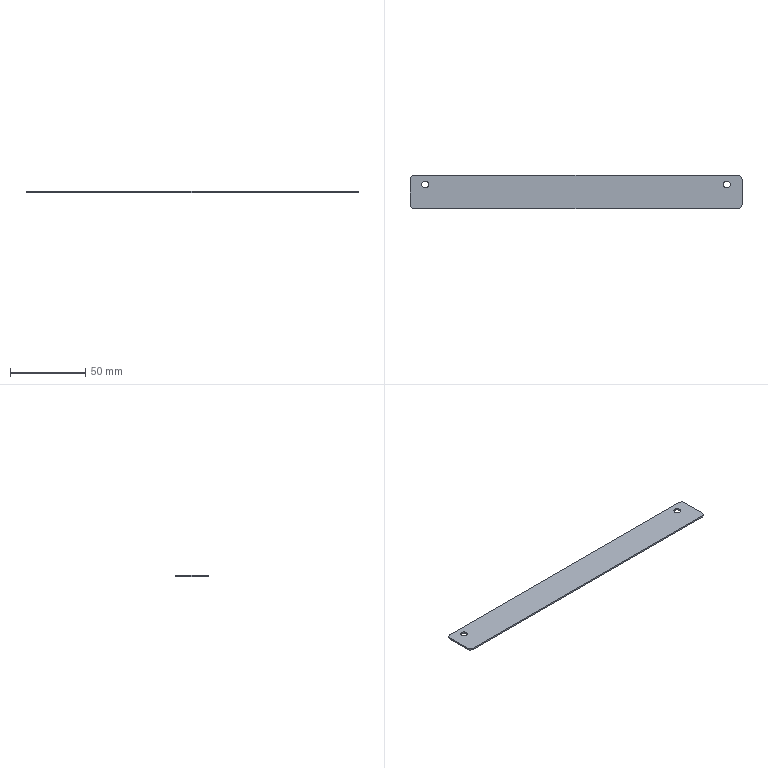Part | STEP file | TY.NE-0002-01-017A Keyboard press block-dddeger | 1 solid | 14 faces | box 220 x 22 x 1 mm | volume 4800 mm3 | cylinder 8 | plane 6 | commonest cylinder face diameters 4.5 x4 6 x4
STEP:
#1=CARTESIAN_POINT('',(0.,0.,0.));
#2=DIRECTION('',(0.,0.,1.));
#3=DIRECTION('',(1.,0.,0.));
#4=AXIS2_PLACEMENT_3D('',#1,#2,#3);
#5=CARTESIAN_POINT('',(102.25,5.,-1.));
#6=VERTEX_POINT('',#5);
#7=CARTESIAN_POINT('',(102.25,5.,0.));
#8=VERTEX_POINT('',#7);
#9=CARTESIAN_POINT('',(102.25,5.,-1.));
#10=DIRECTION('',(0.,0.,1.));
#11=VECTOR('',#10,1.);
#12=LINE('',#9,#11);
#13=CARTESIAN_POINT('',(100.,5.,-1.));
#14=DIRECTION('',(0.,0.,1.));
#15=DIRECTION('',(1.,0.,0.));
#16=AXIS2_PLACEMENT_3D('',#13,#14,#15);
#17=CYLINDRICAL_SURFACE('',#16,2.25);
#18=CARTESIAN_POINT('',(6.283,0.));
#19=DIRECTION('',(0.,1.));
#20=VECTOR('',#19,1.);
#21=LINE('',#18,#20);
#22=(GEOMETRIC_REPRESENTATION_CONTEXT(2)PARAMETRIC_REPRESENTATION_CONTEXT()REPRESENTATION_CONTEXT('',''));
#23=DEFINITIONAL_REPRESENTATION('',(#21),#22);
#24=PCURVE('',#17,#23);
#25=CARTESIAN_POINT('',(100.,5.,-1.));
#26=DIRECTION('',(0.,0.,1.));
#27=DIRECTION('',(1.,0.,0.));
#28=AXIS2_PLACEMENT_3D('',#25,#26,#27);
#29=CYLINDRICAL_SURFACE('',#28,2.25);
#30=CARTESIAN_POINT('',(0.,0.));
#31=DIRECTION('',(0.,1.));
#32=VECTOR('',#31,1.);
#33=LINE('',#30,#32);
#34=(GEOMETRIC_REPRESENTATION_CONTEXT(2)PARAMETRIC_REPRESENTATION_CONTEXT()REPRESENTATION_CONTEXT('',''));
#35=DEFINITIONAL_REPRESENTATION('',(#33),#34);
#36=PCURVE('',#29,#35);
#37=SURFACE_CURVE('',#12,(#24,#36),.PCURVE_S1.);
#38=EDGE_CURVE('',#6,#8,#37,.T.);
#39=ORIENTED_EDGE('',*,*,#38,.T.);
#40=CARTESIAN_POINT('',(97.75,5.,0.));
#41=VERTEX_POINT('',#40);
#42=CARTESIAN_POINT('',(100.,5.,0.));
#43=DIRECTION('',(0.,0.,1.));
#44=DIRECTION('',(-1.,0.,0.));
#45=AXIS2_PLACEMENT_3D('',#42,#43,#44);
#46=CIRCLE('',#45,2.25);
#47=CARTESIAN_POINT('',(3.142,1.));
#48=DIRECTION('',(1.,0.));
#49=VECTOR('',#48,1.);
#50=LINE('',#47,#49);
#51=(GEOMETRIC_REPRESENTATION_CONTEXT(2)PARAMETRIC_REPRESENTATION_CONTEXT()REPRESENTATION_CONTEXT('',''));
#52=DEFINITIONAL_REPRESENTATION('',(#50),#51);
#53=PCURVE('',#17,#52);
#54=CARTESIAN_POINT('',(0.,0.,0.));
#55=DIRECTION('',(0.,0.,1.));
#56=DIRECTION('',(1.,0.,0.));
#57=AXIS2_PLACEMENT_3D('',#54,#55,#56);
#58=PLANE('',#57);
#59=CARTESIAN_POINT('',(100.,5.));
#60=DIRECTION('',(-1.,0.));
#61=AXIS2_PLACEMENT_2D('',#59,#60);
#62=CIRCLE('',#61,2.25);
#63=(GEOMETRIC_REPRESENTATION_CONTEXT(2)PARAMETRIC_REPRESENTATION_CONTEXT()REPRESENTATION_CONTEXT('',''));
#64=DEFINITIONAL_REPRESENTATION('',(#62),#63);
#65=PCURVE('',#58,#64);
#66=SURFACE_CURVE('',#46,(#53,#65),.PCURVE_S1.);
#67=EDGE_CURVE('',#41,#8,#66,.T.);
#68=ORIENTED_EDGE('',*,*,#67,.F.);
#69=CARTESIAN_POINT('',(97.75,5.,-1.));
#70=VERTEX_POINT('',#69);
#71=CARTESIAN_POINT('',(97.75,5.,-1.));
#72=DIRECTION('',(0.,0.,1.));
#73=VECTOR('',#72,1.);
#74=LINE('',#71,#73);
#75=CARTESIAN_POINT('',(3.142,0.));
#76=DIRECTION('',(0.,1.));
#77=VECTOR('',#76,1.);
#78=LINE('',#75,#77);
#79=(GEOMETRIC_REPRESENTATION_CONTEXT(2)PARAMETRIC_REPRESENTATION_CONTEXT()REPRESENTATION_CONTEXT('',''));
#80=DEFINITIONAL_REPRESENTATION('',(#78),#79);
#81=PCURVE('',#17,#80);
#82=CARTESIAN_POINT('',(3.142,0.));
#83=DIRECTION('',(0.,1.));
#84=VECTOR('',#83,1.);
#85=LINE('',#82,#84);
#86=(GEOMETRIC_REPRESENTATION_CONTEXT(2)PARAMETRIC_REPRESENTATION_CONTEXT()REPRESENTATION_CONTEXT('',''));
#87=DEFINITIONAL_REPRESENTATION('',(#85),#86);
#88=PCURVE('',#29,#87);
#89=SURFACE_CURVE('',#74,(#81,#88),.PCURVE_S1.);
#90=EDGE_CURVE('',#70,#41,#89,.T.);
#91=ORIENTED_EDGE('',*,*,#90,.F.);
#92=CARTESIAN_POINT('',(100.,5.,-1.));
#93=DIRECTION('',(0.,0.,1.));
#94=DIRECTION('',(-1.,0.,0.));
#95=AXIS2_PLACEMENT_3D('',#92,#93,#94);
#96=CIRCLE('',#95,2.25);
#97=CARTESIAN_POINT('',(3.142,0.));
#98=DIRECTION('',(1.,0.));
#99=VECTOR('',#98,1.);
#100=LINE('',#97,#99);
#101=(GEOMETRIC_REPRESENTATION_CONTEXT(2)PARAMETRIC_REPRESENTATION_CONTEXT()REPRESENTATION_CONTEXT('',''));
#102=DEFINITIONAL_REPRESENTATION('',(#100),#101);
#103=PCURVE('',#17,#102);
#104=CARTESIAN_POINT('',(0.,0.,-1.));
#105=DIRECTION('',(0.,0.,1.));
#106=DIRECTION('',(1.,0.,0.));
#107=AXIS2_PLACEMENT_3D('',#104,#105,#106);
#108=PLANE('',#107);
#109=CARTESIAN_POINT('',(100.,5.));
#110=DIRECTION('',(-1.,0.));
#111=AXIS2_PLACEMENT_2D('',#109,#110);
#112=CIRCLE('',#111,2.25);
#113=(GEOMETRIC_REPRESENTATION_CONTEXT(2)PARAMETRIC_REPRESENTATION_CONTEXT()REPRESENTATION_CONTEXT('',''));
#114=DEFINITIONAL_REPRESENTATION('',(#112),#113);
#115=PCURVE('',#108,#114);
#116=SURFACE_CURVE('',#96,(#103,#115),.PCURVE_S1.);
#117=EDGE_CURVE('',#70,#6,#116,.T.);
#118=ORIENTED_EDGE('',*,*,#117,.T.);
#119=EDGE_LOOP('',(#39,#68,#91,#118));
#120=FACE_BOUND('',#119,.F.);
#121=ADVANCED_FACE('',(#120),#17,.F.);
#122=CARTESIAN_POINT('',(-97.75,5.,-1.));
#123=VERTEX_POINT('',#122);
#124=CARTESIAN_POINT('',(-97.75,5.,0.));
#125=VERTEX_POINT('',#124);
#126=CARTESIAN_POINT('',(-97.75,5.,-1.));
#127=DIRECTION('',(0.,0.,1.));
#128=VECTOR('',#127,1.);
#129=LINE('',#126,#128);
#130=CARTESIAN_POINT('',(-100.,5.,-1.));
#131=DIRECTION('',(0.,0.,1.));
#132=DIRECTION('',(1.,0.,0.));
#133=AXIS2_PLACEMENT_3D('',#130,#131,#132);
#134=CYLINDRICAL_SURFACE('',#133,2.25);
#135=CARTESIAN_POINT('',(6.283,0.));
#136=DIRECTION('',(0.,1.));
#137=VECTOR('',#136,1.);
#138=LINE('',#135,#137);
#139=(GEOMETRIC_REPRESENTATION_CONTEXT(2)PARAMETRIC_REPRESENTATION_CONTEXT()REPRESENTATION_CONTEXT('',''));
#140=DEFINITIONAL_REPRESENTATION('',(#138),#139);
#141=PCURVE('',#134,#140);
#142=CARTESIAN_POINT('',(-100.,5.,-1.));
#143=DIRECTION('',(0.,0.,1.));
#144=DIRECTION('',(1.,0.,0.));
#145=AXIS2_PLACEMENT_3D('',#142,#143,#144);
#146=CYLINDRICAL_SURFACE('',#145,2.25);
#147=CARTESIAN_POINT('',(0.,0.));
#148=DIRECTION('',(0.,1.));
#149=VECTOR('',#148,1.);
#150=LINE('',#147,#149);
#151=(GEOMETRIC_REPRESENTATION_CONTEXT(2)PARAMETRIC_REPRESENTATION_CONTEXT()REPRESENTATION_CONTEXT('',''));
#152=DEFINITIONAL_REPRESENTATION('',(#150),#151);
#153=PCURVE('',#146,#152);
#154=SURFACE_CURVE('',#129,(#141,#153),.PCURVE_S1.);
#155=EDGE_CURVE('',#123,#125,#154,.T.);
#156=ORIENTED_EDGE('',*,*,#155,.T.);
#157=CARTESIAN_POINT('',(-102.25,5.,0.));
#158=VERTEX_POINT('',#157);
#159=CARTESIAN_POINT('',(-100.,5.,0.));
#160=DIRECTION('',(0.,0.,1.));
#161=DIRECTION('',(1.,0.,0.));
#162=AXIS2_PLACEMENT_3D('',#159,#160,#161);
#163=CIRCLE('',#162,2.25);
#164=CARTESIAN_POINT('',(0.,1.));
#165=DIRECTION('',(1.,0.));
#166=VECTOR('',#165,1.);
#167=LINE('',#164,#166);
#168=(GEOMETRIC_REPRESENTATION_CONTEXT(2)PARAMETRIC_REPRESENTATION_CONTEXT()REPRESENTATION_CONTEXT('',''));
#169=DEFINITIONAL_REPRESENTATION('',(#167),#168);
#170=PCURVE('',#134,#169);
#171=CARTESIAN_POINT('',(-100.,5.));
#172=DIRECTION('',(1.,0.));
#173=AXIS2_PLACEMENT_2D('',#171,#172);
#174=CIRCLE('',#173,2.25);
#175=(GEOMETRIC_REPRESENTATION_CONTEXT(2)PARAMETRIC_REPRESENTATION_CONTEXT()REPRESENTATION_CONTEXT('',''));
#176=DEFINITIONAL_REPRESENTATION('',(#174),#175);
#177=PCURVE('',#58,#176);
#178=SURFACE_CURVE('',#163,(#170,#177),.PCURVE_S1.);
#179=EDGE_CURVE('',#158,#125,#178,.T.);
#180=ORIENTED_EDGE('',*,*,#179,.F.);
#181=CARTESIAN_POINT('',(-102.25,5.,-1.));
#182=VERTEX_POINT('',#181);
#183=CARTESIAN_POINT('',(-102.25,5.,-1.));
#184=DIRECTION('',(0.,0.,1.));
#185=VECTOR('',#184,1.);
#186=LINE('',#183,#185);
#187=CARTESIAN_POINT('',(3.142,0.));
#188=DIRECTION('',(0.,1.));
#189=VECTOR('',#188,1.);
#190=LINE('',#187,#189);
#191=(GEOMETRIC_REPRESENTATION_CONTEXT(2)PARAMETRIC_REPRESENTATION_CONTEXT()REPRESENTATION_CONTEXT('',''));
#192=DEFINITIONAL_REPRESENTATION('',(#190),#191);
#193=PCURVE('',#134,#192);
#194=CARTESIAN_POINT('',(3.142,0.));
#195=DIRECTION('',(0.,1.));
#196=VECTOR('',#195,1.);
#197=LINE('',#194,#196);
#198=(GEOMETRIC_REPRESENTATION_CONTEXT(2)PARAMETRIC_REPRESENTATION_CONTEXT()REPRESENTATION_CONTEXT('',''));
#199=DEFINITIONAL_REPRESENTATION('',(#197),#198);
#200=PCURVE('',#146,#199);
#201=SURFACE_CURVE('',#186,(#193,#200),.PCURVE_S1.);
#202=EDGE_CURVE('',#182,#158,#201,.T.);
#203=ORIENTED_EDGE('',*,*,#202,.F.);
#204=CARTESIAN_POINT('',(-100.,5.,-1.));
#205=DIRECTION('',(0.,0.,1.));
#206=DIRECTION('',(1.,0.,0.));
#207=AXIS2_PLACEMENT_3D('',#204,#205,#206);
#208=CIRCLE('',#207,2.25);
#209=CARTESIAN_POINT('',(0.,0.));
#210=DIRECTION('',(1.,0.));
#211=VECTOR('',#210,1.);
#212=LINE('',#209,#211);
#213=(GEOMETRIC_REPRESENTATION_CONTEXT(2)PARAMETRIC_REPRESENTATION_CONTEXT()REPRESENTATION_CONTEXT('',''));
#214=DEFINITIONAL_REPRESENTATION('',(#212),#213);
#215=PCURVE('',#134,#214);
#216=CARTESIAN_POINT('',(-100.,5.));
#217=DIRECTION('',(1.,0.));
#218=AXIS2_PLACEMENT_2D('',#216,#217);
#219=CIRCLE('',#218,2.25);
#220=(GEOMETRIC_REPRESENTATION_CONTEXT(2)PARAMETRIC_REPRESENTATION_CONTEXT()REPRESENTATION_CONTEXT('',''));
#221=DEFINITIONAL_REPRESENTATION('',(#219),#220);
#222=PCURVE('',#108,#221);
#223=SURFACE_CURVE('',#208,(#215,#222),.PCURVE_S1.);
#224=EDGE_CURVE('',#182,#123,#223,.T.);
#225=ORIENTED_EDGE('',*,*,#224,.T.);
#226=EDGE_LOOP('',(#156,#180,#203,#225));
#227=FACE_BOUND('',#226,.F.);
#228=ADVANCED_FACE('',(#227),#134,.F.);
#229=CARTESIAN_POINT('',(-110.,8.,-1.));
#230=VERTEX_POINT('',#229);
#231=CARTESIAN_POINT('',(-110.,-8.,-1.));
#232=VERTEX_POINT('',#231);
#233=CARTESIAN_POINT('',(-110.,-11.,-1.));
#234=DIRECTION('',(0.,-1.,0.));
#235=VECTOR('',#234,1.);
#236=LINE('',#233,#235);
#237=CARTESIAN_POINT('',(-110.,-11.,-1.));
#238=DIRECTION('',(-1.,0.,0.));
#239=DIRECTION('',(0.,0.,1.));
#240=AXIS2_PLACEMENT_3D('',#237,#238,#239);
#241=PLANE('',#240);
#242=CARTESIAN_POINT('',(0.,0.));
#243=DIRECTION('',(0.,-1.));
#244=VECTOR('',#243,1.);
#245=LINE('',#242,#244);
#246=(GEOMETRIC_REPRESENTATION_CONTEXT(2)PARAMETRIC_REPRESENTATION_CONTEXT()REPRESENTATION_CONTEXT('',''));
#247=DEFINITIONAL_REPRESENTATION('',(#245),#246);
#248=PCURVE('',#241,#247);
#249=CARTESIAN_POINT('',(-110.,-11.));
#250=DIRECTION('',(0.,-1.));
#251=VECTOR('',#250,1.);
#252=LINE('',#249,#251);
#253=(GEOMETRIC_REPRESENTATION_CONTEXT(2)PARAMETRIC_REPRESENTATION_CONTEXT()REPRESENTATION_CONTEXT('',''));
#254=DEFINITIONAL_REPRESENTATION('',(#252),#253);
#255=PCURVE('',#108,#254);
#256=SURFACE_CURVE('',#236,(#248,#255),.PCURVE_S1.);
#257=EDGE_CURVE('',#230,#232,#256,.T.);
#258=ORIENTED_EDGE('',*,*,#257,.T.);
#259=CARTESIAN_POINT('',(-110.,-8.,0.));
#260=VERTEX_POINT('',#259);
#261=CARTESIAN_POINT('',(-110.,-8.,-1.));
#262=DIRECTION('',(0.,0.,1.));
#263=VECTOR('',#262,1.);
#264=LINE('',#261,#263);
#265=CARTESIAN_POINT('',(0.,3.));
#266=DIRECTION('',(1.,0.));
#267=VECTOR('',#266,1.);
#268=LINE('',#265,#267);
#269=(GEOMETRIC_REPRESENTATION_CONTEXT(2)PARAMETRIC_REPRESENTATION_CONTEXT()REPRESENTATION_CONTEXT('',''));
#270=DEFINITIONAL_REPRESENTATION('',(#268),#269);
#271=PCURVE('',#241,#270);
#272=CARTESIAN_POINT('',(-107.,-8.,-1.));
#273=DIRECTION('',(0.,0.,1.));
#274=DIRECTION('',(1.,0.,0.));
#275=AXIS2_PLACEMENT_3D('',#272,#273,#274);
#276=CYLINDRICAL_SURFACE('',#275,3.);
#277=CARTESIAN_POINT('',(3.142,0.));
#278=DIRECTION('',(0.,1.));
#279=VECTOR('',#278,1.);
#280=LINE('',#277,#279);
#281=(GEOMETRIC_REPRESENTATION_CONTEXT(2)PARAMETRIC_REPRESENTATION_CONTEXT()REPRESENTATION_CONTEXT('',''));
#282=DEFINITIONAL_REPRESENTATION('',(#280),#281);
#283=PCURVE('',#276,#282);
#284=SURFACE_CURVE('',#264,(#271,#283),.PCURVE_S1.);
#285=EDGE_CURVE('',#232,#260,#284,.T.);
#286=ORIENTED_EDGE('',*,*,#285,.T.);
#287=CARTESIAN_POINT('',(-110.,8.,0.));
#288=VERTEX_POINT('',#287);
#289=CARTESIAN_POINT('',(-110.,-11.,0.));
#290=DIRECTION('',(0.,-1.,0.));
#291=VECTOR('',#290,1.);
#292=LINE('',#289,#291);
#293=CARTESIAN_POINT('',(1.,0.));
#294=DIRECTION('',(0.,-1.));
#295=VECTOR('',#294,1.);
#296=LINE('',#293,#295);
#297=(GEOMETRIC_REPRESENTATION_CONTEXT(2)PARAMETRIC_REPRESENTATION_CONTEXT()REPRESENTATION_CONTEXT('',''));
#298=DEFINITIONAL_REPRESENTATION('',(#296),#297);
#299=PCURVE('',#241,#298);
#300=CARTESIAN_POINT('',(-110.,-11.));
#301=DIRECTION('',(0.,-1.));
#302=VECTOR('',#301,1.);
#303=LINE('',#300,#302);
#304=(GEOMETRIC_REPRESENTATION_CONTEXT(2)PARAMETRIC_REPRESENTATION_CONTEXT()REPRESENTATION_CONTEXT('',''));
#305=DEFINITIONAL_REPRESENTATION('',(#303),#304);
#306=PCURVE('',#58,#305);
#307=SURFACE_CURVE('',#292,(#299,#306),.PCURVE_S1.);
#308=EDGE_CURVE('',#288,#260,#307,.T.);
#309=ORIENTED_EDGE('',*,*,#308,.F.);
#310=CARTESIAN_POINT('',(-110.,8.,-1.));
#311=DIRECTION('',(0.,0.,-1.));
#312=VECTOR('',#311,1.);
#313=LINE('',#310,#312);
#314=CARTESIAN_POINT('',(0.,19.));
#315=DIRECTION('',(-1.,0.));
#316=VECTOR('',#315,1.);
#317=LINE('',#314,#316);
#318=(GEOMETRIC_REPRESENTATION_CONTEXT(2)PARAMETRIC_REPRESENTATION_CONTEXT()REPRESENTATION_CONTEXT('',''));
#319=DEFINITIONAL_REPRESENTATION('',(#317),#318);
#320=PCURVE('',#241,#319);
#321=CARTESIAN_POINT('',(-107.,8.,-1.));
#322=DIRECTION('',(0.,0.,1.));
#323=DIRECTION('',(1.,0.,0.));
#324=AXIS2_PLACEMENT_3D('',#321,#322,#323);
#325=CYLINDRICAL_SURFACE('',#324,3.);
#326=CARTESIAN_POINT('',(3.142,0.));
#327=DIRECTION('',(0.,-1.));
#328=VECTOR('',#327,1.);
#329=LINE('',#326,#328);
#330=(GEOMETRIC_REPRESENTATION_CONTEXT(2)PARAMETRIC_REPRESENTATION_CONTEXT()REPRESENTATION_CONTEXT('',''));
#331=DEFINITIONAL_REPRESENTATION('',(#329),#330);
#332=PCURVE('',#325,#331);
#333=SURFACE_CURVE('',#313,(#320,#332),.PCURVE_S1.);
#334=EDGE_CURVE('',#288,#230,#333,.T.);
#335=ORIENTED_EDGE('',*,*,#334,.T.);
#336=EDGE_LOOP('',(#258,#286,#309,#335));
#337=FACE_BOUND('',#336,.T.);
#338=ADVANCED_FACE('',(#337),#241,.T.);
#339=CARTESIAN_POINT('',(107.,11.,-1.));
#340=VERTEX_POINT('',#339);
#341=CARTESIAN_POINT('',(-107.,11.,-1.));
#342=VERTEX_POINT('',#341);
#343=CARTESIAN_POINT('',(110.,11.,-1.));
#344=DIRECTION('',(-1.,0.,0.));
#345=VECTOR('',#344,1.);
#346=LINE('',#343,#345);
#347=CARTESIAN_POINT('',(110.,11.,-1.));
#348=DIRECTION('',(0.,1.,0.));
#349=DIRECTION('',(-1.,0.,0.));
#350=AXIS2_PLACEMENT_3D('',#347,#348,#349);
#351=PLANE('',#350);
#352=CARTESIAN_POINT('',(0.,0.));
#353=DIRECTION('',(1.,0.));
#354=VECTOR('',#353,1.);
#355=LINE('',#352,#354);
#356=(GEOMETRIC_REPRESENTATION_CONTEXT(2)PARAMETRIC_REPRESENTATION_CONTEXT()REPRESENTATION_CONTEXT('',''));
#357=DEFINITIONAL_REPRESENTATION('',(#355),#356);
#358=PCURVE('',#351,#357);
#359=CARTESIAN_POINT('',(110.,11.));
#360=DIRECTION('',(-1.,0.));
#361=VECTOR('',#360,1.);
#362=LINE('',#359,#361);
#363=(GEOMETRIC_REPRESENTATION_CONTEXT(2)PARAMETRIC_REPRESENTATION_CONTEXT()REPRESENTATION_CONTEXT('',''));
#364=DEFINITIONAL_REPRESENTATION('',(#362),#363);
#365=PCURVE('',#108,#364);
#366=SURFACE_CURVE('',#346,(#358,#365),.PCURVE_S1.);
#367=EDGE_CURVE('',#340,#342,#366,.T.);
#368=ORIENTED_EDGE('',*,*,#367,.T.);
#369=CARTESIAN_POINT('',(-107.,11.,0.));
#370=VERTEX_POINT('',#369);
#371=CARTESIAN_POINT('',(-107.,11.,-1.));
#372=DIRECTION('',(0.,0.,1.));
#373=VECTOR('',#372,1.);
#374=LINE('',#371,#373);
#375=CARTESIAN_POINT('',(217.,0.));
#376=DIRECTION('',(0.,1.));
#377=VECTOR('',#376,1.);
#378=LINE('',#375,#377);
#379=(GEOMETRIC_REPRESENTATION_CONTEXT(2)PARAMETRIC_REPRESENTATION_CONTEXT()REPRESENTATION_CONTEXT('',''));
#380=DEFINITIONAL_REPRESENTATION('',(#378),#379);
#381=PCURVE('',#351,#380);
#382=CARTESIAN_POINT('',(1.571,0.));
#383=DIRECTION('',(0.,1.));
#384=VECTOR('',#383,1.);
#385=LINE('',#382,#384);
#386=(GEOMETRIC_REPRESENTATION_CONTEXT(2)PARAMETRIC_REPRESENTATION_CONTEXT()REPRESENTATION_CONTEXT('',''));
#387=DEFINITIONAL_REPRESENTATION('',(#385),#386);
#388=PCURVE('',#325,#387);
#389=SURFACE_CURVE('',#374,(#381,#388),.PCURVE_S1.);
#390=EDGE_CURVE('',#342,#370,#389,.T.);
#391=ORIENTED_EDGE('',*,*,#390,.T.);
#392=CARTESIAN_POINT('',(107.,11.,0.));
#393=VERTEX_POINT('',#392);
#394=CARTESIAN_POINT('',(110.,11.,0.));
#395=DIRECTION('',(-1.,0.,0.));
#396=VECTOR('',#395,1.);
#397=LINE('',#394,#396);
#398=CARTESIAN_POINT('',(0.,1.));
#399=DIRECTION('',(1.,0.));
#400=VECTOR('',#399,1.);
#401=LINE('',#398,#400);
#402=(GEOMETRIC_REPRESENTATION_CONTEXT(2)PARAMETRIC_REPRESENTATION_CONTEXT()REPRESENTATION_CONTEXT('',''));
#403=DEFINITIONAL_REPRESENTATION('',(#401),#402);
#404=PCURVE('',#351,#403);
#405=CARTESIAN_POINT('',(110.,11.));
#406=DIRECTION('',(-1.,0.));
#407=VECTOR('',#406,1.);
#408=LINE('',#405,#407);
#409=(GEOMETRIC_REPRESENTATION_CONTEXT(2)PARAMETRIC_REPRESENTATION_CONTEXT()REPRESENTATION_CONTEXT('',''));
#410=DEFINITIONAL_REPRESENTATION('',(#408),#409);
#411=PCURVE('',#58,#410);
#412=SURFACE_CURVE('',#397,(#404,#411),.PCURVE_S1.);
#413=EDGE_CURVE('',#393,#370,#412,.T.);
#414=ORIENTED_EDGE('',*,*,#413,.F.);
#415=CARTESIAN_POINT('',(107.,11.,-1.));
#416=DIRECTION('',(0.,0.,-1.));
#417=VECTOR('',#416,1.);
#418=LINE('',#415,#417);
#419=CARTESIAN_POINT('',(3.,0.));
#420=DIRECTION('',(0.,-1.));
#421=VECTOR('',#420,1.);
#422=LINE('',#419,#421);
#423=(GEOMETRIC_REPRESENTATION_CONTEXT(2)PARAMETRIC_REPRESENTATION_CONTEXT()REPRESENTATION_CONTEXT('',''));
#424=DEFINITIONAL_REPRESENTATION('',(#422),#423);
#425=PCURVE('',#351,#424);
#426=CARTESIAN_POINT('',(107.,8.,-1.));
#427=DIRECTION('',(0.,0.,1.));
#428=DIRECTION('',(1.,0.,0.));
#429=AXIS2_PLACEMENT_3D('',#426,#427,#428);
#430=CYLINDRICAL_SURFACE('',#429,3.);
#431=CARTESIAN_POINT('',(1.571,0.));
#432=DIRECTION('',(0.,-1.));
#433=VECTOR('',#432,1.);
#434=LINE('',#431,#433);
#435=(GEOMETRIC_REPRESENTATION_CONTEXT(2)PARAMETRIC_REPRESENTATION_CONTEXT()REPRESENTATION_CONTEXT('',''));
#436=DEFINITIONAL_REPRESENTATION('',(#434),#435);
#437=PCURVE('',#430,#436);
#438=SURFACE_CURVE('',#418,(#425,#437),.PCURVE_S1.);
#439=EDGE_CURVE('',#393,#340,#438,.T.);
#440=ORIENTED_EDGE('',*,*,#439,.T.);
#441=EDGE_LOOP('',(#368,#391,#414,#440));
#442=FACE_BOUND('',#441,.T.);
#443=ADVANCED_FACE('',(#442),#351,.T.);
#444=CARTESIAN_POINT('',(110.,-8.,0.));
#445=VERTEX_POINT('',#444);
#446=CARTESIAN_POINT('',(110.,8.,0.));
#447=VERTEX_POINT('',#446);
#448=CARTESIAN_POINT('',(110.,-11.,0.));
#449=DIRECTION('',(0.,1.,0.));
#450=VECTOR('',#449,1.);
#451=LINE('',#448,#450);
#452=CARTESIAN_POINT('',(110.,-11.,-1.));
#453=DIRECTION('',(1.,0.,0.));
#454=DIRECTION('',(0.,0.,-1.));
#455=AXIS2_PLACEMENT_3D('',#452,#453,#454);
#456=PLANE('',#455);
#457=CARTESIAN_POINT('',(-1.,0.));
#458=DIRECTION('',(0.,1.));
#459=VECTOR('',#458,1.);
#460=LINE('',#457,#459);
#461=(GEOMETRIC_REPRESENTATION_CONTEXT(2)PARAMETRIC_REPRESENTATION_CONTEXT()REPRESENTATION_CONTEXT('',''));
#462=DEFINITIONAL_REPRESENTATION('',(#460),#461);
#463=PCURVE('',#456,#462);
#464=CARTESIAN_POINT('',(110.,-11.));
#465=DIRECTION('',(0.,1.));
#466=VECTOR('',#465,1.);
#467=LINE('',#464,#466);
#468=(GEOMETRIC_REPRESENTATION_CONTEXT(2)PARAMETRIC_REPRESENTATION_CONTEXT()REPRESENTATION_CONTEXT('',''));
#469=DEFINITIONAL_REPRESENTATION('',(#467),#468);
#470=PCURVE('',#58,#469);
#471=SURFACE_CURVE('',#451,(#463,#470),.PCURVE_S1.);
#472=EDGE_CURVE('',#445,#447,#471,.T.);
#473=ORIENTED_EDGE('',*,*,#472,.F.);
#474=CARTESIAN_POINT('',(110.,-8.,-1.));
#475=VERTEX_POINT('',#474);
#476=CARTESIAN_POINT('',(110.,-8.,-1.));
#477=DIRECTION('',(0.,0.,-1.));
#478=VECTOR('',#477,1.);
#479=LINE('',#476,#478);
#480=CARTESIAN_POINT('',(0.,3.));
#481=DIRECTION('',(1.,0.));
#482=VECTOR('',#481,1.);
#483=LINE('',#480,#482);
#484=(GEOMETRIC_REPRESENTATION_CONTEXT(2)PARAMETRIC_REPRESENTATION_CONTEXT()REPRESENTATION_CONTEXT('',''));
#485=DEFINITIONAL_REPRESENTATION('',(#483),#484);
#486=PCURVE('',#456,#485);
#487=CARTESIAN_POINT('',(107.,-8.,-1.));
#488=DIRECTION('',(0.,0.,1.));
#489=DIRECTION('',(1.,0.,0.));
#490=AXIS2_PLACEMENT_3D('',#487,#488,#489);
#491=CYLINDRICAL_SURFACE('',#490,3.);
#492=CARTESIAN_POINT('',(6.283,0.));
#493=DIRECTION('',(0.,-1.));
#494=VECTOR('',#493,1.);
#495=LINE('',#492,#494);
#496=(GEOMETRIC_REPRESENTATION_CONTEXT(2)PARAMETRIC_REPRESENTATION_CONTEXT()REPRESENTATION_CONTEXT('',''));
#497=DEFINITIONAL_REPRESENTATION('',(#495),#496);
#498=PCURVE('',#491,#497);
#499=SURFACE_CURVE('',#479,(#486,#498),.PCURVE_S1.);
#500=EDGE_CURVE('',#445,#475,#499,.T.);
#501=ORIENTED_EDGE('',*,*,#500,.T.);
#502=CARTESIAN_POINT('',(110.,8.,-1.));
#503=VERTEX_POINT('',#502);
#504=CARTESIAN_POINT('',(110.,-11.,-1.));
#505=DIRECTION('',(0.,1.,0.));
#506=VECTOR('',#505,1.);
#507=LINE('',#504,#506);
#508=CARTESIAN_POINT('',(0.,0.));
#509=DIRECTION('',(0.,1.));
#510=VECTOR('',#509,1.);
#511=LINE('',#508,#510);
#512=(GEOMETRIC_REPRESENTATION_CONTEXT(2)PARAMETRIC_REPRESENTATION_CONTEXT()REPRESENTATION_CONTEXT('',''));
#513=DEFINITIONAL_REPRESENTATION('',(#511),#512);
#514=PCURVE('',#456,#513);
#515=CARTESIAN_POINT('',(110.,-11.));
#516=DIRECTION('',(0.,1.));
#517=VECTOR('',#516,1.);
#518=LINE('',#515,#517);
#519=(GEOMETRIC_REPRESENTATION_CONTEXT(2)PARAMETRIC_REPRESENTATION_CONTEXT()REPRESENTATION_CONTEXT('',''));
#520=DEFINITIONAL_REPRESENTATION('',(#518),#519);
#521=PCURVE('',#108,#520);
#522=SURFACE_CURVE('',#507,(#514,#521),.PCURVE_S1.);
#523=EDGE_CURVE('',#475,#503,#522,.T.);
#524=ORIENTED_EDGE('',*,*,#523,.T.);
#525=CARTESIAN_POINT('',(110.,8.,-1.));
#526=DIRECTION('',(0.,0.,1.));
#527=VECTOR('',#526,1.);
#528=LINE('',#525,#527);
#529=CARTESIAN_POINT('',(0.,19.));
#530=DIRECTION('',(-1.,0.));
#531=VECTOR('',#530,1.);
#532=LINE('',#529,#531);
#533=(GEOMETRIC_REPRESENTATION_CONTEXT(2)PARAMETRIC_REPRESENTATION_CONTEXT()REPRESENTATION_CONTEXT('',''));
#534=DEFINITIONAL_REPRESENTATION('',(#532),#533);
#535=PCURVE('',#456,#534);
#536=CARTESIAN_POINT('',(0.,0.));
#537=DIRECTION('',(0.,1.));
#538=VECTOR('',#537,1.);
#539=LINE('',#536,#538);
#540=(GEOMETRIC_REPRESENTATION_CONTEXT(2)PARAMETRIC_REPRESENTATION_CONTEXT()REPRESENTATION_CONTEXT('',''));
#541=DEFINITIONAL_REPRESENTATION('',(#539),#540);
#542=PCURVE('',#430,#541);
#543=SURFACE_CURVE('',#528,(#535,#542),.PCURVE_S1.);
#544=EDGE_CURVE('',#503,#447,#543,.T.);
#545=ORIENTED_EDGE('',*,*,#544,.T.);
#546=EDGE_LOOP('',(#473,#501,#524,#545));
#547=FACE_BOUND('',#546,.T.);
#548=ADVANCED_FACE('',(#547),#456,.T.);
#549=CARTESIAN_POINT('',(-107.,-11.,0.));
#550=VERTEX_POINT('',#549);
#551=CARTESIAN_POINT('',(107.,-11.,0.));
#552=VERTEX_POINT('',#551);
#553=CARTESIAN_POINT('',(110.,-11.,0.));
#554=DIRECTION('',(1.,0.,0.));
#555=VECTOR('',#554,1.);
#556=LINE('',#553,#555);
#557=CARTESIAN_POINT('',(110.,-11.,-1.));
#558=DIRECTION('',(0.,-1.,0.));
#559=DIRECTION('',(1.,0.,0.));
#560=AXIS2_PLACEMENT_3D('',#557,#558,#559);
#561=PLANE('',#560);
#562=CARTESIAN_POINT('',(0.,1.));
#563=DIRECTION('',(1.,0.));
#564=VECTOR('',#563,1.);
#565=LINE('',#562,#564);
#566=(GEOMETRIC_REPRESENTATION_CONTEXT(2)PARAMETRIC_REPRESENTATION_CONTEXT()REPRESENTATION_CONTEXT('',''));
#567=DEFINITIONAL_REPRESENTATION('',(#565),#566);
#568=PCURVE('',#561,#567);
#569=CARTESIAN_POINT('',(110.,-11.));
#570=DIRECTION('',(1.,0.));
#571=VECTOR('',#570,1.);
#572=LINE('',#569,#571);
#573=(GEOMETRIC_REPRESENTATION_CONTEXT(2)PARAMETRIC_REPRESENTATION_CONTEXT()REPRESENTATION_CONTEXT('',''));
#574=DEFINITIONAL_REPRESENTATION('',(#572),#573);
#575=PCURVE('',#58,#574);
#576=SURFACE_CURVE('',#556,(#568,#575),.PCURVE_S1.);
#577=EDGE_CURVE('',#550,#552,#576,.T.);
#578=ORIENTED_EDGE('',*,*,#577,.F.);
#579=CARTESIAN_POINT('',(-107.,-11.,-1.));
#580=VERTEX_POINT('',#579);
#581=CARTESIAN_POINT('',(-107.,-11.,-1.));
#582=DIRECTION('',(0.,0.,-1.));
#583=VECTOR('',#582,1.);
#584=LINE('',#581,#583);
#585=CARTESIAN_POINT('',(-217.,0.));
#586=DIRECTION('',(0.,-1.));
#587=VECTOR('',#586,1.);
#588=LINE('',#585,#587);
#589=(GEOMETRIC_REPRESENTATION_CONTEXT(2)PARAMETRIC_REPRESENTATION_CONTEXT()REPRESENTATION_CONTEXT('',''));
#590=DEFINITIONAL_REPRESENTATION('',(#588),#589);
#591=PCURVE('',#561,#590);
#592=CARTESIAN_POINT('',(4.712,0.));
#593=DIRECTION('',(0.,-1.));
#594=VECTOR('',#593,1.);
#595=LINE('',#592,#594);
#596=(GEOMETRIC_REPRESENTATION_CONTEXT(2)PARAMETRIC_REPRESENTATION_CONTEXT()REPRESENTATION_CONTEXT('',''));
#597=DEFINITIONAL_REPRESENTATION('',(#595),#596);
#598=PCURVE('',#276,#597);
#599=SURFACE_CURVE('',#584,(#591,#598),.PCURVE_S1.);
#600=EDGE_CURVE('',#550,#580,#599,.T.);
#601=ORIENTED_EDGE('',*,*,#600,.T.);
#602=CARTESIAN_POINT('',(107.,-11.,-1.));
#603=VERTEX_POINT('',#602);
#604=CARTESIAN_POINT('',(110.,-11.,-1.));
#605=DIRECTION('',(1.,0.,0.));
#606=VECTOR('',#605,1.);
#607=LINE('',#604,#606);
#608=CARTESIAN_POINT('',(0.,0.));
#609=DIRECTION('',(1.,0.));
#610=VECTOR('',#609,1.);
#611=LINE('',#608,#610);
#612=(GEOMETRIC_REPRESENTATION_CONTEXT(2)PARAMETRIC_REPRESENTATION_CONTEXT()REPRESENTATION_CONTEXT('',''));
#613=DEFINITIONAL_REPRESENTATION('',(#611),#612);
#614=PCURVE('',#561,#613);
#615=CARTESIAN_POINT('',(110.,-11.));
#616=DIRECTION('',(1.,0.));
#617=VECTOR('',#616,1.);
#618=LINE('',#615,#617);
#619=(GEOMETRIC_REPRESENTATION_CONTEXT(2)PARAMETRIC_REPRESENTATION_CONTEXT()REPRESENTATION_CONTEXT('',''));
#620=DEFINITIONAL_REPRESENTATION('',(#618),#619);
#621=PCURVE('',#108,#620);
#622=SURFACE_CURVE('',#607,(#614,#621),.PCURVE_S1.);
#623=EDGE_CURVE('',#580,#603,#622,.T.);
#624=ORIENTED_EDGE('',*,*,#623,.T.);
#625=CARTESIAN_POINT('',(107.,-11.,-1.));
#626=DIRECTION('',(0.,0.,1.));
#627=VECTOR('',#626,1.);
#628=LINE('',#625,#627);
#629=CARTESIAN_POINT('',(-3.,0.));
#630=DIRECTION('',(0.,1.));
#631=VECTOR('',#630,1.);
#632=LINE('',#629,#631);
#633=(GEOMETRIC_REPRESENTATION_CONTEXT(2)PARAMETRIC_REPRESENTATION_CONTEXT()REPRESENTATION_CONTEXT('',''));
#634=DEFINITIONAL_REPRESENTATION('',(#632),#633);
#635=PCURVE('',#561,#634);
#636=CARTESIAN_POINT('',(4.712,0.));
#637=DIRECTION('',(0.,1.));
#638=VECTOR('',#637,1.);
#639=LINE('',#636,#638);
#640=(GEOMETRIC_REPRESENTATION_CONTEXT(2)PARAMETRIC_REPRESENTATION_CONTEXT()REPRESENTATION_CONTEXT('',''));
#641=DEFINITIONAL_REPRESENTATION('',(#639),#640);
#642=PCURVE('',#491,#641);
#643=SURFACE_CURVE('',#628,(#635,#642),.PCURVE_S1.);
#644=EDGE_CURVE('',#603,#552,#643,.T.);
#645=ORIENTED_EDGE('',*,*,#644,.T.);
#646=EDGE_LOOP('',(#578,#601,#624,#645));
#647=FACE_BOUND('',#646,.T.);
#648=ADVANCED_FACE('',(#647),#561,.T.);
#649=CARTESIAN_POINT('',(100.,5.,-1.));
#650=DIRECTION('',(0.,0.,1.));
#651=DIRECTION('',(-1.,0.,0.));
#652=AXIS2_PLACEMENT_3D('',#649,#650,#651);
#653=CIRCLE('',#652,2.25);
#654=CARTESIAN_POINT('',(100.,5.));
#655=DIRECTION('',(-1.,0.));
#656=AXIS2_PLACEMENT_2D('',#654,#655);
#657=CIRCLE('',#656,2.25);
#658=(GEOMETRIC_REPRESENTATION_CONTEXT(2)PARAMETRIC_REPRESENTATION_CONTEXT()REPRESENTATION_CONTEXT('',''));
#659=DEFINITIONAL_REPRESENTATION('',(#657),#658);
#660=PCURVE('',#108,#659);
#661=CARTESIAN_POINT('',(-3.142,0.));
#662=DIRECTION('',(1.,0.));
#663=VECTOR('',#662,1.);
#664=LINE('',#661,#663);
#665=(GEOMETRIC_REPRESENTATION_CONTEXT(2)PARAMETRIC_REPRESENTATION_CONTEXT()REPRESENTATION_CONTEXT('',''));
#666=DEFINITIONAL_REPRESENTATION('',(#664),#665);
#667=PCURVE('',#29,#666);
#668=SURFACE_CURVE('',#653,(#660,#667),.PCURVE_S1.);
#669=EDGE_CURVE('',#6,#70,#668,.T.);
#670=ORIENTED_EDGE('',*,*,#669,.T.);
#671=ORIENTED_EDGE('',*,*,#117,.T.);
#672=EDGE_LOOP('',(#670,#671));
#673=FACE_BOUND('',#672,.T.);
#674=CARTESIAN_POINT('',(-100.,5.,-1.));
#675=DIRECTION('',(0.,0.,1.));
#676=DIRECTION('',(1.,0.,0.));
#677=AXIS2_PLACEMENT_3D('',#674,#675,#676);
#678=CIRCLE('',#677,2.25);
#679=CARTESIAN_POINT('',(-100.,5.));
#680=DIRECTION('',(1.,0.));
#681=AXIS2_PLACEMENT_2D('',#679,#680);
#682=CIRCLE('',#681,2.25);
#683=(GEOMETRIC_REPRESENTATION_CONTEXT(2)PARAMETRIC_REPRESENTATION_CONTEXT()REPRESENTATION_CONTEXT('',''));
#684=DEFINITIONAL_REPRESENTATION('',(#682),#683);
#685=PCURVE('',#108,#684);
#686=CARTESIAN_POINT('',(0.,0.));
#687=DIRECTION('',(1.,0.));
#688=VECTOR('',#687,1.);
#689=LINE('',#686,#688);
#690=(GEOMETRIC_REPRESENTATION_CONTEXT(2)PARAMETRIC_REPRESENTATION_CONTEXT()REPRESENTATION_CONTEXT('',''));
#691=DEFINITIONAL_REPRESENTATION('',(#689),#690);
#692=PCURVE('',#146,#691);
#693=SURFACE_CURVE('',#678,(#685,#692),.PCURVE_S1.);
#694=EDGE_CURVE('',#123,#182,#693,.T.);
#695=ORIENTED_EDGE('',*,*,#694,.T.);
#696=ORIENTED_EDGE('',*,*,#224,.T.);
#697=EDGE_LOOP('',(#695,#696));
#698=FACE_BOUND('',#697,.T.);
#699=ORIENTED_EDGE('',*,*,#623,.F.);
#700=CARTESIAN_POINT('',(-107.,-8.,-1.));
#701=DIRECTION('',(0.,0.,-1.));
#702=DIRECTION('',(1.,0.,0.));
#703=AXIS2_PLACEMENT_3D('',#700,#701,#702);
#704=CIRCLE('',#703,3.);
#705=CARTESIAN_POINT('',(-104.,-8.));
#706=CARTESIAN_POINT('',(-104.,-13.196));
#707=CARTESIAN_POINT('',(-108.5,-10.598));
#708=CARTESIAN_POINT('',(-113.,-8.));
#709=CARTESIAN_POINT('',(-108.5,-5.402));
#710=CARTESIAN_POINT('',(-104.,-2.804));
#711=CARTESIAN_POINT('',(-104.,-8.));
#712=(BOUNDED_CURVE()B_SPLINE_CURVE(2,(#705,#706,#707,#708,#709,#710,#711),.UNSPECIFIED.,.T.,.F.)B_SPLINE_CURVE_WITH_KNOTS((1,2,2,2,2,1),(-2.094,0.,2.094,4.189,6.283,8.378),.UNSPECIFIED.)CURVE()GEOMETRIC_REPRESENTATION_ITEM()RATIONAL_B_SPLINE_CURVE((1.,0.5,1.,0.5,1.,0.5,1.))REPRESENTATION_ITEM(''));
#713=(GEOMETRIC_REPRESENTATION_CONTEXT(2)PARAMETRIC_REPRESENTATION_CONTEXT()REPRESENTATION_CONTEXT('',''));
#714=DEFINITIONAL_REPRESENTATION('',(#712),#713);
#715=PCURVE('',#108,#714);
#716=CARTESIAN_POINT('',(6.283,0.));
#717=DIRECTION('',(-1.,0.));
#718=VECTOR('',#717,1.);
#719=LINE('',#716,#718);
#720=(GEOMETRIC_REPRESENTATION_CONTEXT(2)PARAMETRIC_REPRESENTATION_CONTEXT()REPRESENTATION_CONTEXT('',''));
#721=DEFINITIONAL_REPRESENTATION('',(#719),#720);
#722=PCURVE('',#276,#721);
#723=SURFACE_CURVE('',#704,(#715,#722),.PCURVE_S1.);
#724=EDGE_CURVE('',#580,#232,#723,.T.);
#725=ORIENTED_EDGE('',*,*,#724,.T.);
#726=ORIENTED_EDGE('',*,*,#257,.F.);
#727=CARTESIAN_POINT('',(-107.,8.,-1.));
#728=DIRECTION('',(0.,0.,-1.));
#729=DIRECTION('',(1.,0.,0.));
#730=AXIS2_PLACEMENT_3D('',#727,#728,#729);
#731=CIRCLE('',#730,3.);
#732=CARTESIAN_POINT('',(-104.,8.));
#733=CARTESIAN_POINT('',(-104.,2.804));
#734=CARTESIAN_POINT('',(-108.5,5.402));
#735=CARTESIAN_POINT('',(-113.,8.));
#736=CARTESIAN_POINT('',(-108.5,10.598));
#737=CARTESIAN_POINT('',(-104.,13.196));
#738=CARTESIAN_POINT('',(-104.,8.));
#739=(BOUNDED_CURVE()B_SPLINE_CURVE(2,(#732,#733,#734,#735,#736,#737,#738),.UNSPECIFIED.,.T.,.F.)B_SPLINE_CURVE_WITH_KNOTS((1,2,2,2,2,1),(-2.094,0.,2.094,4.189,6.283,8.378),.UNSPECIFIED.)CURVE()GEOMETRIC_REPRESENTATION_ITEM()RATIONAL_B_SPLINE_CURVE((1.,0.5,1.,0.5,1.,0.5,1.))REPRESENTATION_ITEM(''));
#740=(GEOMETRIC_REPRESENTATION_CONTEXT(2)PARAMETRIC_REPRESENTATION_CONTEXT()REPRESENTATION_CONTEXT('',''));
#741=DEFINITIONAL_REPRESENTATION('',(#739),#740);
#742=PCURVE('',#108,#741);
#743=CARTESIAN_POINT('',(6.283,0.));
#744=DIRECTION('',(-1.,0.));
#745=VECTOR('',#744,1.);
#746=LINE('',#743,#745);
#747=(GEOMETRIC_REPRESENTATION_CONTEXT(2)PARAMETRIC_REPRESENTATION_CONTEXT()REPRESENTATION_CONTEXT('',''));
#748=DEFINITIONAL_REPRESENTATION('',(#746),#747);
#749=PCURVE('',#325,#748);
#750=SURFACE_CURVE('',#731,(#742,#749),.PCURVE_S1.);
#751=EDGE_CURVE('',#230,#342,#750,.T.);
#752=ORIENTED_EDGE('',*,*,#751,.T.);
#753=ORIENTED_EDGE('',*,*,#367,.F.);
#754=CARTESIAN_POINT('',(107.,8.,-1.));
#755=DIRECTION('',(0.,0.,-1.));
#756=DIRECTION('',(1.,0.,0.));
#757=AXIS2_PLACEMENT_3D('',#754,#755,#756);
#758=CIRCLE('',#757,3.);
#759=CARTESIAN_POINT('',(110.,8.));
#760=CARTESIAN_POINT('',(110.,2.804));
#761=CARTESIAN_POINT('',(105.5,5.402));
#762=CARTESIAN_POINT('',(101.,8.));
#763=CARTESIAN_POINT('',(105.5,10.598));
#764=CARTESIAN_POINT('',(110.,13.196));
#765=CARTESIAN_POINT('',(110.,8.));
#766=(BOUNDED_CURVE()B_SPLINE_CURVE(2,(#759,#760,#761,#762,#763,#764,#765),.UNSPECIFIED.,.T.,.F.)B_SPLINE_CURVE_WITH_KNOTS((1,2,2,2,2,1),(-2.094,0.,2.094,4.189,6.283,8.378),.UNSPECIFIED.)CURVE()GEOMETRIC_REPRESENTATION_ITEM()RATIONAL_B_SPLINE_CURVE((1.,0.5,1.,0.5,1.,0.5,1.))REPRESENTATION_ITEM(''));
#767=(GEOMETRIC_REPRESENTATION_CONTEXT(2)PARAMETRIC_REPRESENTATION_CONTEXT()REPRESENTATION_CONTEXT('',''));
#768=DEFINITIONAL_REPRESENTATION('',(#766),#767);
#769=PCURVE('',#108,#768);
#770=CARTESIAN_POINT('',(6.283,0.));
#771=DIRECTION('',(-1.,0.));
#772=VECTOR('',#771,1.);
#773=LINE('',#770,#772);
#774=(GEOMETRIC_REPRESENTATION_CONTEXT(2)PARAMETRIC_REPRESENTATION_CONTEXT()REPRESENTATION_CONTEXT('',''));
#775=DEFINITIONAL_REPRESENTATION('',(#773),#774);
#776=PCURVE('',#430,#775);
#777=SURFACE_CURVE('',#758,(#769,#776),.PCURVE_S1.);
#778=EDGE_CURVE('',#340,#503,#777,.T.);
#779=ORIENTED_EDGE('',*,*,#778,.T.);
#780=ORIENTED_EDGE('',*,*,#523,.F.);
#781=CARTESIAN_POINT('',(107.,-8.,-1.));
#782=DIRECTION('',(0.,0.,-1.));
#783=DIRECTION('',(1.,0.,0.));
#784=AXIS2_PLACEMENT_3D('',#781,#782,#783);
#785=CIRCLE('',#784,3.);
#786=CARTESIAN_POINT('',(110.,-8.));
#787=CARTESIAN_POINT('',(110.,-13.196));
#788=CARTESIAN_POINT('',(105.5,-10.598));
#789=CARTESIAN_POINT('',(101.,-8.));
#790=CARTESIAN_POINT('',(105.5,-5.402));
#791=CARTESIAN_POINT('',(110.,-2.804));
#792=CARTESIAN_POINT('',(110.,-8.));
#793=(BOUNDED_CURVE()B_SPLINE_CURVE(2,(#786,#787,#788,#789,#790,#791,#792),.UNSPECIFIED.,.T.,.F.)B_SPLINE_CURVE_WITH_KNOTS((1,2,2,2,2,1),(-2.094,0.,2.094,4.189,6.283,8.378),.UNSPECIFIED.)CURVE()GEOMETRIC_REPRESENTATION_ITEM()RATIONAL_B_SPLINE_CURVE((1.,0.5,1.,0.5,1.,0.5,1.))REPRESENTATION_ITEM(''));
#794=(GEOMETRIC_REPRESENTATION_CONTEXT(2)PARAMETRIC_REPRESENTATION_CONTEXT()REPRESENTATION_CONTEXT('',''));
#795=DEFINITIONAL_REPRESENTATION('',(#793),#794);
#796=PCURVE('',#108,#795);
#797=CARTESIAN_POINT('',(6.283,0.));
#798=DIRECTION('',(-1.,0.));
#799=VECTOR('',#798,1.);
#800=LINE('',#797,#799);
#801=(GEOMETRIC_REPRESENTATION_CONTEXT(2)PARAMETRIC_REPRESENTATION_CONTEXT()REPRESENTATION_CONTEXT('',''));
#802=DEFINITIONAL_REPRESENTATION('',(#800),#801);
#803=PCURVE('',#491,#802);
#804=SURFACE_CURVE('',#785,(#796,#803),.PCURVE_S1.);
#805=EDGE_CURVE('',#475,#603,#804,.T.);
#806=ORIENTED_EDGE('',*,*,#805,.T.);
#807=EDGE_LOOP('',(#699,#725,#726,#752,#753,#779,#780,#806));
#808=FACE_BOUND('',#807,.T.);
#809=ADVANCED_FACE('',(#673,#698,#808),#108,.F.);
#810=CARTESIAN_POINT('',(100.,5.,0.));
#811=DIRECTION('',(0.,0.,1.));
#812=DIRECTION('',(-1.,0.,0.));
#813=AXIS2_PLACEMENT_3D('',#810,#811,#812);
#814=CIRCLE('',#813,2.25);
#815=CARTESIAN_POINT('',(100.,5.));
#816=DIRECTION('',(-1.,0.));
#817=AXIS2_PLACEMENT_2D('',#815,#816);
#818=CIRCLE('',#817,2.25);
#819=(GEOMETRIC_REPRESENTATION_CONTEXT(2)PARAMETRIC_REPRESENTATION_CONTEXT()REPRESENTATION_CONTEXT('',''));
#820=DEFINITIONAL_REPRESENTATION('',(#818),#819);
#821=PCURVE('',#58,#820);
#822=CARTESIAN_POINT('',(-3.142,1.));
#823=DIRECTION('',(1.,0.));
#824=VECTOR('',#823,1.);
#825=LINE('',#822,#824);
#826=(GEOMETRIC_REPRESENTATION_CONTEXT(2)PARAMETRIC_REPRESENTATION_CONTEXT()REPRESENTATION_CONTEXT('',''));
#827=DEFINITIONAL_REPRESENTATION('',(#825),#826);
#828=PCURVE('',#29,#827);
#829=SURFACE_CURVE('',#814,(#821,#828),.PCURVE_S1.);
#830=EDGE_CURVE('',#8,#41,#829,.T.);
#831=ORIENTED_EDGE('',*,*,#830,.F.);
#832=ORIENTED_EDGE('',*,*,#67,.F.);
#833=EDGE_LOOP('',(#831,#832));
#834=FACE_BOUND('',#833,.T.);
#835=CARTESIAN_POINT('',(-100.,5.,0.));
#836=DIRECTION('',(0.,0.,1.));
#837=DIRECTION('',(1.,0.,0.));
#838=AXIS2_PLACEMENT_3D('',#835,#836,#837);
#839=CIRCLE('',#838,2.25);
#840=CARTESIAN_POINT('',(-100.,5.));
#841=DIRECTION('',(1.,0.));
#842=AXIS2_PLACEMENT_2D('',#840,#841);
#843=CIRCLE('',#842,2.25);
#844=(GEOMETRIC_REPRESENTATION_CONTEXT(2)PARAMETRIC_REPRESENTATION_CONTEXT()REPRESENTATION_CONTEXT('',''));
#845=DEFINITIONAL_REPRESENTATION('',(#843),#844);
#846=PCURVE('',#58,#845);
#847=CARTESIAN_POINT('',(0.,1.));
#848=DIRECTION('',(1.,0.));
#849=VECTOR('',#848,1.);
#850=LINE('',#847,#849);
#851=(GEOMETRIC_REPRESENTATION_CONTEXT(2)PARAMETRIC_REPRESENTATION_CONTEXT()REPRESENTATION_CONTEXT('',''));
#852=DEFINITIONAL_REPRESENTATION('',(#850),#851);
#853=PCURVE('',#146,#852);
#854=SURFACE_CURVE('',#839,(#846,#853),.PCURVE_S1.);
#855=EDGE_CURVE('',#125,#158,#854,.T.);
#856=ORIENTED_EDGE('',*,*,#855,.F.);
#857=ORIENTED_EDGE('',*,*,#179,.F.);
#858=EDGE_LOOP('',(#856,#857));
#859=FACE_BOUND('',#858,.T.);
#860=ORIENTED_EDGE('',*,*,#308,.T.);
#861=CARTESIAN_POINT('',(-107.,-8.,0.));
#862=DIRECTION('',(0.,0.,1.));
#863=DIRECTION('',(1.,0.,0.));
#864=AXIS2_PLACEMENT_3D('',#861,#862,#863);
#865=CIRCLE('',#864,3.);
#866=CARTESIAN_POINT('',(-107.,-8.));
#867=DIRECTION('',(1.,0.));
#868=AXIS2_PLACEMENT_2D('',#866,#867);
#869=CIRCLE('',#868,3.);
#870=(GEOMETRIC_REPRESENTATION_CONTEXT(2)PARAMETRIC_REPRESENTATION_CONTEXT()REPRESENTATION_CONTEXT('',''));
#871=DEFINITIONAL_REPRESENTATION('',(#869),#870);
#872=PCURVE('',#58,#871);
#873=CARTESIAN_POINT('',(0.,1.));
#874=DIRECTION('',(1.,0.));
#875=VECTOR('',#874,1.);
#876=LINE('',#873,#875);
#877=(GEOMETRIC_REPRESENTATION_CONTEXT(2)PARAMETRIC_REPRESENTATION_CONTEXT()REPRESENTATION_CONTEXT('',''));
#878=DEFINITIONAL_REPRESENTATION('',(#876),#877);
#879=PCURVE('',#276,#878);
#880=SURFACE_CURVE('',#865,(#872,#879),.PCURVE_S1.);
#881=EDGE_CURVE('',#260,#550,#880,.T.);
#882=ORIENTED_EDGE('',*,*,#881,.T.);
#883=ORIENTED_EDGE('',*,*,#577,.T.);
#884=CARTESIAN_POINT('',(107.,-8.,0.));
#885=DIRECTION('',(0.,0.,1.));
#886=DIRECTION('',(1.,0.,0.));
#887=AXIS2_PLACEMENT_3D('',#884,#885,#886);
#888=CIRCLE('',#887,3.);
#889=CARTESIAN_POINT('',(107.,-8.));
#890=DIRECTION('',(1.,0.));
#891=AXIS2_PLACEMENT_2D('',#889,#890);
#892=CIRCLE('',#891,3.);
#893=(GEOMETRIC_REPRESENTATION_CONTEXT(2)PARAMETRIC_REPRESENTATION_CONTEXT()REPRESENTATION_CONTEXT('',''));
#894=DEFINITIONAL_REPRESENTATION('',(#892),#893);
#895=PCURVE('',#58,#894);
#896=CARTESIAN_POINT('',(0.,1.));
#897=DIRECTION('',(1.,0.));
#898=VECTOR('',#897,1.);
#899=LINE('',#896,#898);
#900=(GEOMETRIC_REPRESENTATION_CONTEXT(2)PARAMETRIC_REPRESENTATION_CONTEXT()REPRESENTATION_CONTEXT('',''));
#901=DEFINITIONAL_REPRESENTATION('',(#899),#900);
#902=PCURVE('',#491,#901);
#903=SURFACE_CURVE('',#888,(#895,#902),.PCURVE_S1.);
#904=EDGE_CURVE('',#552,#445,#903,.T.);
#905=ORIENTED_EDGE('',*,*,#904,.T.);
#906=ORIENTED_EDGE('',*,*,#472,.T.);
#907=CARTESIAN_POINT('',(107.,8.,0.));
#908=DIRECTION('',(0.,0.,1.));
#909=DIRECTION('',(1.,0.,0.));
#910=AXIS2_PLACEMENT_3D('',#907,#908,#909);
#911=CIRCLE('',#910,3.);
#912=CARTESIAN_POINT('',(107.,8.));
#913=DIRECTION('',(1.,0.));
#914=AXIS2_PLACEMENT_2D('',#912,#913);
#915=CIRCLE('',#914,3.);
#916=(GEOMETRIC_REPRESENTATION_CONTEXT(2)PARAMETRIC_REPRESENTATION_CONTEXT()REPRESENTATION_CONTEXT('',''));
#917=DEFINITIONAL_REPRESENTATION('',(#915),#916);
#918=PCURVE('',#58,#917);
#919=CARTESIAN_POINT('',(0.,1.));
#920=DIRECTION('',(1.,0.));
#921=VECTOR('',#920,1.);
#922=LINE('',#919,#921);
#923=(GEOMETRIC_REPRESENTATION_CONTEXT(2)PARAMETRIC_REPRESENTATION_CONTEXT()REPRESENTATION_CONTEXT('',''));
#924=DEFINITIONAL_REPRESENTATION('',(#922),#923);
#925=PCURVE('',#430,#924);
#926=SURFACE_CURVE('',#911,(#918,#925),.PCURVE_S1.);
#927=EDGE_CURVE('',#447,#393,#926,.T.);
#928=ORIENTED_EDGE('',*,*,#927,.T.);
#929=ORIENTED_EDGE('',*,*,#413,.T.);
#930=CARTESIAN_POINT('',(-107.,8.,0.));
#931=DIRECTION('',(0.,0.,1.));
#932=DIRECTION('',(1.,0.,0.));
#933=AXIS2_PLACEMENT_3D('',#930,#931,#932);
#934=CIRCLE('',#933,3.);
#935=CARTESIAN_POINT('',(-107.,8.));
#936=DIRECTION('',(1.,0.));
#937=AXIS2_PLACEMENT_2D('',#935,#936);
#938=CIRCLE('',#937,3.);
#939=(GEOMETRIC_REPRESENTATION_CONTEXT(2)PARAMETRIC_REPRESENTATION_CONTEXT()REPRESENTATION_CONTEXT('',''));
#940=DEFINITIONAL_REPRESENTATION('',(#938),#939);
#941=PCURVE('',#58,#940);
#942=CARTESIAN_POINT('',(0.,1.));
#943=DIRECTION('',(1.,0.));
#944=VECTOR('',#943,1.);
#945=LINE('',#942,#944);
#946=(GEOMETRIC_REPRESENTATION_CONTEXT(2)PARAMETRIC_REPRESENTATION_CONTEXT()REPRESENTATION_CONTEXT('',''));
#947=DEFINITIONAL_REPRESENTATION('',(#945),#946);
#948=PCURVE('',#325,#947);
#949=SURFACE_CURVE('',#934,(#941,#948),.PCURVE_S1.);
#950=EDGE_CURVE('',#370,#288,#949,.T.);
#951=ORIENTED_EDGE('',*,*,#950,.T.);
#952=EDGE_LOOP('',(#860,#882,#883,#905,#906,#928,#929,#951));
#953=FACE_BOUND('',#952,.T.);
#954=ADVANCED_FACE('',(#834,#859,#953),#58,.T.);
#955=ORIENTED_EDGE('',*,*,#855,.F.);
#956=ORIENTED_EDGE('',*,*,#155,.F.);
#957=ORIENTED_EDGE('',*,*,#694,.T.);
#958=ORIENTED_EDGE('',*,*,#202,.T.);
#959=EDGE_LOOP('',(#955,#956,#957,#958));
#960=FACE_BOUND('',#959,.F.);
#961=ADVANCED_FACE('',(#960),#146,.F.);
#962=ORIENTED_EDGE('',*,*,#830,.F.);
#963=ORIENTED_EDGE('',*,*,#38,.F.);
#964=ORIENTED_EDGE('',*,*,#669,.T.);
#965=ORIENTED_EDGE('',*,*,#90,.T.);
#966=EDGE_LOOP('',(#962,#963,#964,#965));
#967=FACE_BOUND('',#966,.F.);
#968=ADVANCED_FACE('',(#967),#29,.F.);
#969=ORIENTED_EDGE('',*,*,#724,.F.);
#970=ORIENTED_EDGE('',*,*,#600,.F.);
#971=ORIENTED_EDGE('',*,*,#881,.F.);
#972=ORIENTED_EDGE('',*,*,#285,.F.);
#973=EDGE_LOOP('',(#969,#970,#971,#972));
#974=FACE_BOUND('',#973,.T.);
#975=ADVANCED_FACE('',(#974),#276,.T.);
#976=ORIENTED_EDGE('',*,*,#805,.F.);
#977=ORIENTED_EDGE('',*,*,#500,.F.);
#978=ORIENTED_EDGE('',*,*,#904,.F.);
#979=ORIENTED_EDGE('',*,*,#644,.F.);
#980=EDGE_LOOP('',(#976,#977,#978,#979));
#981=FACE_BOUND('',#980,.T.);
#982=ADVANCED_FACE('',(#981),#491,.T.);
#983=ORIENTED_EDGE('',*,*,#751,.F.);
#984=ORIENTED_EDGE('',*,*,#334,.F.);
#985=ORIENTED_EDGE('',*,*,#950,.F.);
#986=ORIENTED_EDGE('',*,*,#390,.F.);
#987=EDGE_LOOP('',(#983,#984,#985,#986));
#988=FACE_BOUND('',#987,.T.);
#989=ADVANCED_FACE('',(#988),#325,.T.);
#990=ORIENTED_EDGE('',*,*,#778,.F.);
#991=ORIENTED_EDGE('',*,*,#439,.F.);
#992=ORIENTED_EDGE('',*,*,#927,.F.);
#993=ORIENTED_EDGE('',*,*,#544,.F.);
#994=EDGE_LOOP('',(#990,#991,#992,#993));
#995=FACE_BOUND('',#994,.T.);
#996=ADVANCED_FACE('',(#995),#430,.T.);
#997=CLOSED_SHELL('',(#121,#228,#338,#443,#548,#648,#809,#954,#961,#968,#975,#982,#989,#996));
#998=MANIFOLD_SOLID_BREP('',#997);
#999=(LENGTH_UNIT()NAMED_UNIT(*)SI_UNIT(.MILLI.,.METRE.));
#1000=UNCERTAINTY_MEASURE_WITH_UNIT(LENGTH_MEASURE(0.0000001),#999,'','');
#1001=(NAMED_UNIT(*)PLANE_ANGLE_UNIT()SI_UNIT($,.RADIAN.));
#1002=(NAMED_UNIT(*)SI_UNIT($,.STERADIAN.)SOLID_ANGLE_UNIT());
#1003=(GEOMETRIC_REPRESENTATION_CONTEXT(3)GLOBAL_UNCERTAINTY_ASSIGNED_CONTEXT((#1000))GLOBAL_UNIT_ASSIGNED_CONTEXT((#999,#1001,#1002))REPRESENTATION_CONTEXT('',''));
#1004=ADVANCED_BREP_SHAPE_REPRESENTATION('',(#4,#998),#1003);